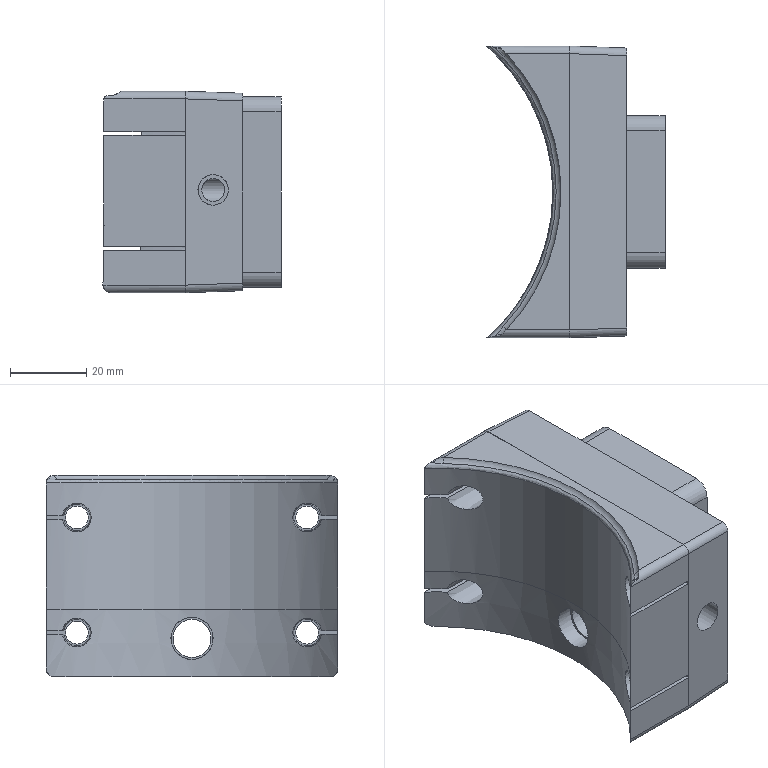Part | NX | features solid 2 | 1 solid | 124 faces | box 46.65 x 76.4 x 52.783 mm | volume 102758 mm3 | plane 62 | cylinder 49 | cone 7 | spline 4 | torus 2 | commonest cylinder face diameters 5 x16 6 x9 8 x7 4 x4 4.02 x4 6.7 x2